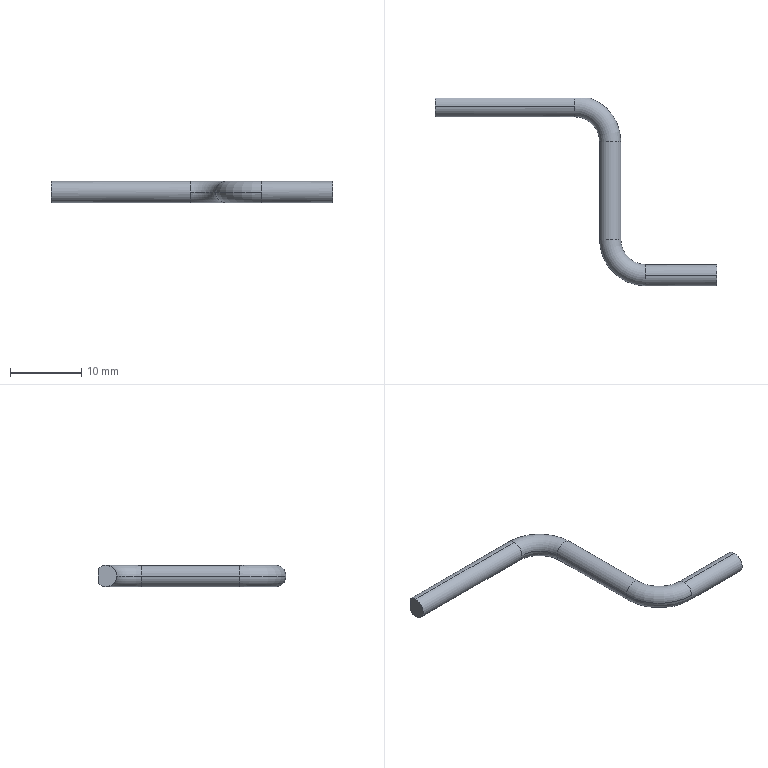Part | SolidWorks | features BaseBody 1 | 1 solid | 14 faces | box 39.607 x 26.395 x 3 mm | volume 406.832 mm3 | cylinder 7 | torus 4 | plane 3 | commonest cylinder face diameters 3 x7
STEP:
#1=CARTESIAN_POINT('',(-28.5,-35.,0.));
#2=VERTEX_POINT('',#1);
#3=CARTESIAN_POINT('',(-31.5,-35.,0.));
#4=VERTEX_POINT('',#3);
#5=CARTESIAN_POINT('',(-30.,-35.,0.));
#6=DIRECTION('',(0.,-1.,0.));
#7=DIRECTION('',(0.,0.,-1.));
#8=AXIS2_PLACEMENT_3D('',#5,#6,#7);
#9=CIRCLE('',#8,1.5);
#10=EDGE_CURVE('',#2,#4,#9,.T.);
#11=ORIENTED_EDGE('',*,*,#10,.T.);
#12=CARTESIAN_POINT('',(-25.,-41.5,0.));
#13=VERTEX_POINT('',#12);
#14=CARTESIAN_POINT('',(-25.,-35.,0.));
#15=DIRECTION('',(0.,0.,1.));
#16=DIRECTION('',(1.,0.,0.));
#17=AXIS2_PLACEMENT_3D('',#14,#15,#16);
#18=CIRCLE('',#17,6.5);
#19=EDGE_CURVE('',#4,#13,#18,.T.);
#20=ORIENTED_EDGE('',*,*,#19,.T.);
#21=CARTESIAN_POINT('',(-25.,-40.,1.5));
#22=VERTEX_POINT('',#21);
#23=CARTESIAN_POINT('',(-25.,-40.,0.));
#24=DIRECTION('',(1.,0.,0.));
#25=DIRECTION('',(0.,0.,-1.));
#26=AXIS2_PLACEMENT_3D('',#23,#24,#25);
#27=CIRCLE('',#26,1.5);
#28=EDGE_CURVE('',#22,#13,#27,.T.);
#29=ORIENTED_EDGE('',*,*,#28,.F.);
#30=CARTESIAN_POINT('',(-25.,-38.5,0.));
#31=VERTEX_POINT('',#30);
#32=CARTESIAN_POINT('',(-25.,-40.,0.));
#33=DIRECTION('',(1.,0.,0.));
#34=DIRECTION('',(0.,0.,-1.));
#35=AXIS2_PLACEMENT_3D('',#32,#33,#34);
#36=CIRCLE('',#35,1.5);
#37=EDGE_CURVE('',#31,#22,#36,.T.);
#38=ORIENTED_EDGE('',*,*,#37,.F.);
#39=CARTESIAN_POINT('',(-25.,-35.,0.));
#40=DIRECTION('',(0.,0.,1.));
#41=DIRECTION('',(1.,0.,0.));
#42=AXIS2_PLACEMENT_3D('',#39,#40,#41);
#43=CIRCLE('',#42,3.5);
#44=EDGE_CURVE('',#2,#31,#43,.T.);
#45=ORIENTED_EDGE('',*,*,#44,.F.);
#46=EDGE_LOOP('',(#11,#20,#29,#38,#45));
#47=FACE_OUTER_BOUND('',#46,.T.);
#48=CARTESIAN_POINT('',(-25.,-35.,0.));
#49=DIRECTION('',(0.,0.,1.));
#50=DIRECTION('',(1.,0.,0.));
#51=AXIS2_PLACEMENT_3D('',#48,#49,#50);
#52=TOROIDAL_SURFACE('',#51,5.,1.5);
#53=ADVANCED_FACE('',(#47),#52,.T.);
#54=CARTESIAN_POINT('',(-32.812,-15.105,0.));
#55=VERTEX_POINT('',#54);
#56=CARTESIAN_POINT('',(-35.,-15.105,-0.9972));
#57=VERTEX_POINT('',#56);
#58=CARTESIAN_POINT('',(-32.812,-15.105,0.));
#59=CARTESIAN_POINT('',(-32.812,-15.105,-0.1106));
#60=CARTESIAN_POINT('',(-32.849,-15.105,-0.2168));
#61=CARTESIAN_POINT('',(-32.968,-15.105,-0.4004));
#62=CARTESIAN_POINT('',(-33.048,-15.105,-0.4771));
#63=CARTESIAN_POINT('',(-33.31,-15.105,-0.6742));
#64=CARTESIAN_POINT('',(-33.512,-15.105,-0.76));
#65=CARTESIAN_POINT('',(-33.927,-15.105,-0.8892));
#66=CARTESIAN_POINT('',(-34.139,-15.105,-0.9304));
#67=CARTESIAN_POINT('',(-34.566,-15.105,-0.9846));
#68=CARTESIAN_POINT('',(-34.784,-15.105,-0.9972));
#69=CARTESIAN_POINT('',(-35.,-15.105,-0.9972));
#70=B_SPLINE_CURVE_WITH_KNOTS('',3,(#58,#59,#60,#61,#62,#63,#64,#65,#66,#67,#68,#69),.UNSPECIFIED.,.F.,.F.,(4,2,2,2,2,4),(0.,0.0003263,0.0006525,0.001305,0.001958,0.00261),.UNSPECIFIED.);
#71=EDGE_CURVE('',#55,#57,#70,.T.);
#72=ORIENTED_EDGE('',*,*,#71,.F.);
#73=CARTESIAN_POINT('',(-28.5,-21.225,0.));
#74=VERTEX_POINT('',#73);
#75=CARTESIAN_POINT('',(-35.,-21.225,0.));
#76=DIRECTION('',(0.,0.,-1.));
#77=DIRECTION('',(-1.,0.,0.));
#78=AXIS2_PLACEMENT_3D('',#75,#76,#77);
#79=CIRCLE('',#78,6.5);
#80=EDGE_CURVE('',#55,#74,#79,.T.);
#81=ORIENTED_EDGE('',*,*,#80,.T.);
#82=CARTESIAN_POINT('',(-31.5,-21.225,0.));
#83=VERTEX_POINT('',#82);
#84=CARTESIAN_POINT('',(-30.,-21.225,0.));
#85=DIRECTION('',(0.,-1.,0.));
#86=DIRECTION('',(0.,0.,-1.));
#87=AXIS2_PLACEMENT_3D('',#84,#85,#86);
#88=CIRCLE('',#87,1.5);
#89=EDGE_CURVE('',#83,#74,#88,.T.);
#90=ORIENTED_EDGE('',*,*,#89,.F.);
#91=CARTESIAN_POINT('',(-35.,-17.725,0.));
#92=VERTEX_POINT('',#91);
#93=CARTESIAN_POINT('',(-35.,-21.225,0.));
#94=DIRECTION('',(0.,0.,-1.));
#95=DIRECTION('',(-1.,0.,0.));
#96=AXIS2_PLACEMENT_3D('',#93,#94,#95);
#97=CIRCLE('',#96,3.5);
#98=EDGE_CURVE('',#92,#83,#97,.T.);
#99=ORIENTED_EDGE('',*,*,#98,.F.);
#100=CARTESIAN_POINT('',(-35.,-16.225,-1.5));
#101=VERTEX_POINT('',#100);
#102=CARTESIAN_POINT('',(-35.,-16.225,0.));
#103=DIRECTION('',(1.,0.,0.));
#104=DIRECTION('',(0.,0.,-1.));
#105=AXIS2_PLACEMENT_3D('',#102,#103,#104);
#106=CIRCLE('',#105,1.5);
#107=EDGE_CURVE('',#92,#101,#106,.T.);
#108=ORIENTED_EDGE('',*,*,#107,.T.);
#109=CARTESIAN_POINT('',(-35.,-16.225,0.));
#110=DIRECTION('',(1.,0.,0.));
#111=DIRECTION('',(0.,0.,-1.));
#112=AXIS2_PLACEMENT_3D('',#109,#110,#111);
#113=CIRCLE('',#112,1.5);
#114=EDGE_CURVE('',#101,#57,#113,.T.);
#115=ORIENTED_EDGE('',*,*,#114,.T.);
#116=EDGE_LOOP('',(#72,#81,#90,#99,#108,#115));
#117=FACE_OUTER_BOUND('',#116,.T.);
#118=CARTESIAN_POINT('',(-35.,-21.225,0.));
#119=DIRECTION('',(0.,0.,-1.));
#120=DIRECTION('',(-1.,0.,0.));
#121=AXIS2_PLACEMENT_3D('',#118,#119,#120);
#122=TOROIDAL_SURFACE('',#121,5.,1.5);
#123=ADVANCED_FACE('',(#117),#122,.T.);
#124=CARTESIAN_POINT('',(-25.,-40.,-1.5));
#125=VERTEX_POINT('',#124);
#126=CARTESIAN_POINT('',(-25.,-40.,0.));
#127=DIRECTION('',(1.,0.,0.));
#128=DIRECTION('',(0.,0.,-1.));
#129=AXIS2_PLACEMENT_3D('',#126,#127,#128);
#130=CIRCLE('',#129,1.5);
#131=EDGE_CURVE('',#125,#31,#130,.T.);
#132=ORIENTED_EDGE('',*,*,#131,.T.);
#133=ORIENTED_EDGE('',*,*,#37,.T.);
#134=CARTESIAN_POINT('',(-15.,-40.,1.5));
#135=VERTEX_POINT('',#134);
#136=CARTESIAN_POINT('',(-25.,-40.,1.5));
#137=DIRECTION('',(1.,0.,0.));
#138=VECTOR('',#137,1000.);
#139=LINE('',#136,#138);
#140=EDGE_CURVE('',#22,#135,#139,.T.);
#141=ORIENTED_EDGE('',*,*,#140,.T.);
#142=CARTESIAN_POINT('',(-15.,-40.,-1.5));
#143=VERTEX_POINT('',#142);
#144=CARTESIAN_POINT('',(-15.,-40.,0.));
#145=DIRECTION('',(1.,0.,0.));
#146=DIRECTION('',(0.,0.,-1.));
#147=AXIS2_PLACEMENT_3D('',#144,#145,#146);
#148=CIRCLE('',#147,1.5);
#149=EDGE_CURVE('',#143,#135,#148,.T.);
#150=ORIENTED_EDGE('',*,*,#149,.F.);
#151=CARTESIAN_POINT('',(-25.,-40.,-1.5));
#152=DIRECTION('',(1.,0.,0.));
#153=VECTOR('',#152,1000.);
#154=LINE('',#151,#153);
#155=EDGE_CURVE('',#125,#143,#154,.T.);
#156=ORIENTED_EDGE('',*,*,#155,.F.);
#157=EDGE_LOOP('',(#132,#133,#141,#150,#156));
#158=FACE_OUTER_BOUND('',#157,.T.);
#159=CARTESIAN_POINT('',(-25.,-40.,0.));
#160=DIRECTION('',(1.,0.,0.));
#161=DIRECTION('',(0.,0.,-1.));
#162=AXIS2_PLACEMENT_3D('',#159,#160,#161);
#163=CYLINDRICAL_SURFACE('',#162,1.5);
#164=ADVANCED_FACE('',(#158),#163,.T.);
#165=CARTESIAN_POINT('',(-30.,-21.225,0.));
#166=DIRECTION('',(0.,-1.,0.));
#167=DIRECTION('',(0.,0.,-1.));
#168=AXIS2_PLACEMENT_3D('',#165,#166,#167);
#169=CIRCLE('',#168,1.5);
#170=EDGE_CURVE('',#74,#83,#169,.T.);
#171=ORIENTED_EDGE('',*,*,#170,.T.);
#172=CARTESIAN_POINT('',(-31.5,-21.225,0.));
#173=DIRECTION('',(0.,-1.,0.));
#174=VECTOR('',#173,1000.);
#175=LINE('',#172,#174);
#176=EDGE_CURVE('',#83,#4,#175,.T.);
#177=ORIENTED_EDGE('',*,*,#176,.T.);
#178=ORIENTED_EDGE('',*,*,#10,.F.);
#179=CARTESIAN_POINT('',(-28.5,-21.225,0.));
#180=DIRECTION('',(0.,-1.,0.));
#181=VECTOR('',#180,1000.);
#182=LINE('',#179,#181);
#183=EDGE_CURVE('',#74,#2,#182,.T.);
#184=ORIENTED_EDGE('',*,*,#183,.F.);
#185=EDGE_LOOP('',(#171,#177,#178,#184));
#186=FACE_OUTER_BOUND('',#185,.T.);
#187=CARTESIAN_POINT('',(-30.,-21.225,0.));
#188=DIRECTION('',(0.,-1.,0.));
#189=DIRECTION('',(1.,0.,0.));
#190=AXIS2_PLACEMENT_3D('',#187,#188,#189);
#191=CYLINDRICAL_SURFACE('',#190,1.5);
#192=ADVANCED_FACE('',(#186),#191,.T.);
#193=CARTESIAN_POINT('',(-54.607,-15.105,0.9972));
#194=VERTEX_POINT('',#193);
#195=CARTESIAN_POINT('',(-54.607,-16.225,1.5));
#196=VERTEX_POINT('',#195);
#197=CARTESIAN_POINT('',(-54.607,-16.225,0.));
#198=DIRECTION('',(1.,0.,0.));
#199=DIRECTION('',(0.,0.,-1.));
#200=AXIS2_PLACEMENT_3D('',#197,#198,#199);
#201=CIRCLE('',#200,1.5);
#202=EDGE_CURVE('',#194,#196,#201,.T.);
#203=ORIENTED_EDGE('',*,*,#202,.T.);
#204=CARTESIAN_POINT('',(-35.,-16.225,1.5));
#205=VERTEX_POINT('',#204);
#206=CARTESIAN_POINT('',(-54.607,-16.225,1.5));
#207=DIRECTION('',(1.,0.,0.));
#208=VECTOR('',#207,1000.);
#209=LINE('',#206,#208);
#210=EDGE_CURVE('',#196,#205,#209,.T.);
#211=ORIENTED_EDGE('',*,*,#210,.T.);
#212=CARTESIAN_POINT('',(-35.,-15.105,0.9972));
#213=VERTEX_POINT('',#212);
#214=CARTESIAN_POINT('',(-35.,-16.225,0.));
#215=DIRECTION('',(1.,0.,0.));
#216=DIRECTION('',(0.,0.,-1.));
#217=AXIS2_PLACEMENT_3D('',#214,#215,#216);
#218=CIRCLE('',#217,1.5);
#219=EDGE_CURVE('',#213,#205,#218,.T.);
#220=ORIENTED_EDGE('',*,*,#219,.F.);
#221=CARTESIAN_POINT('',(-54.607,-15.105,0.9972));
#222=DIRECTION('',(1.,0.,0.));
#223=VECTOR('',#222,1000.);
#224=LINE('',#221,#223);
#225=EDGE_CURVE('',#194,#213,#224,.T.);
#226=ORIENTED_EDGE('',*,*,#225,.F.);
#227=EDGE_LOOP('',(#203,#211,#220,#226));
#228=FACE_OUTER_BOUND('',#227,.T.);
#229=CARTESIAN_POINT('',(-54.607,-16.225,0.));
#230=DIRECTION('',(1.,0.,0.));
#231=DIRECTION('',(0.,0.,-1.));
#232=AXIS2_PLACEMENT_3D('',#229,#230,#231);
#233=CYLINDRICAL_SURFACE('',#232,1.5);
#234=ADVANCED_FACE('',(#228),#233,.T.);
#235=ORIENTED_EDGE('',*,*,#210,.F.);
#236=CARTESIAN_POINT('',(-54.607,-16.225,-1.5));
#237=VERTEX_POINT('',#236);
#238=CARTESIAN_POINT('',(-54.607,-16.225,0.));
#239=DIRECTION('',(1.,0.,0.));
#240=DIRECTION('',(0.,0.,-1.));
#241=AXIS2_PLACEMENT_3D('',#238,#239,#240);
#242=CIRCLE('',#241,1.5);
#243=EDGE_CURVE('',#196,#237,#242,.T.);
#244=ORIENTED_EDGE('',*,*,#243,.T.);
#245=CARTESIAN_POINT('',(-54.607,-16.225,-1.5));
#246=DIRECTION('',(1.,0.,0.));
#247=VECTOR('',#246,1000.);
#248=LINE('',#245,#247);
#249=EDGE_CURVE('',#237,#101,#248,.T.);
#250=ORIENTED_EDGE('',*,*,#249,.T.);
#251=ORIENTED_EDGE('',*,*,#107,.F.);
#252=CARTESIAN_POINT('',(-35.,-16.225,0.));
#253=DIRECTION('',(1.,0.,0.));
#254=DIRECTION('',(0.,0.,-1.));
#255=AXIS2_PLACEMENT_3D('',#252,#253,#254);
#256=CIRCLE('',#255,1.5);
#257=EDGE_CURVE('',#205,#92,#256,.T.);
#258=ORIENTED_EDGE('',*,*,#257,.F.);
#259=EDGE_LOOP('',(#235,#244,#250,#251,#258));
#260=FACE_OUTER_BOUND('',#259,.T.);
#261=CARTESIAN_POINT('',(-54.607,-16.225,0.));
#262=DIRECTION('',(1.,0.,0.));
#263=DIRECTION('',(0.,0.,-1.));
#264=AXIS2_PLACEMENT_3D('',#261,#262,#263);
#265=CYLINDRICAL_SURFACE('',#264,1.5);
#266=ADVANCED_FACE('',(#260),#265,.T.);
#267=ORIENTED_EDGE('',*,*,#202,.F.);
#268=CARTESIAN_POINT('',(-54.607,-15.105,-0.9972));
#269=VERTEX_POINT('',#268);
#270=CARTESIAN_POINT('',(-54.607,-15.105,0.));
#271=DIRECTION('',(0.,0.,-1.));
#272=VECTOR('',#271,1000.);
#273=LINE('',#270,#272);
#274=EDGE_CURVE('',#194,#269,#273,.T.);
#275=ORIENTED_EDGE('',*,*,#274,.T.);
#276=CARTESIAN_POINT('',(-54.607,-16.225,0.));
#277=DIRECTION('',(1.,0.,0.));
#278=DIRECTION('',(0.,0.,-1.));
#279=AXIS2_PLACEMENT_3D('',#276,#277,#278);
#280=CIRCLE('',#279,1.5);
#281=EDGE_CURVE('',#237,#269,#280,.T.);
#282=ORIENTED_EDGE('',*,*,#281,.F.);
#283=ORIENTED_EDGE('',*,*,#243,.F.);
#284=EDGE_LOOP('',(#267,#275,#282,#283));
#285=FACE_OUTER_BOUND('',#284,.T.);
#286=CARTESIAN_POINT('',(-54.607,-16.225,0.));
#287=DIRECTION('',(1.,0.,0.));
#288=DIRECTION('',(0.,0.,-1.));
#289=AXIS2_PLACEMENT_3D('',#286,#287,#288);
#290=PLANE('',#289);
#291=ADVANCED_FACE('',(#285),#290,.F.);
#292=ORIENTED_EDGE('',*,*,#149,.T.);
#293=CARTESIAN_POINT('',(-15.,-40.,0.));
#294=DIRECTION('',(1.,0.,0.));
#295=DIRECTION('',(0.,0.,-1.));
#296=AXIS2_PLACEMENT_3D('',#293,#294,#295);
#297=CIRCLE('',#296,1.5);
#298=EDGE_CURVE('',#135,#143,#297,.T.);
#299=ORIENTED_EDGE('',*,*,#298,.T.);
#300=EDGE_LOOP('',(#292,#299));
#301=FACE_OUTER_BOUND('',#300,.T.);
#302=CARTESIAN_POINT('',(-15.,-40.,0.));
#303=DIRECTION('',(1.,0.,0.));
#304=DIRECTION('',(0.,0.,-1.));
#305=AXIS2_PLACEMENT_3D('',#302,#303,#304);
#306=PLANE('',#305);
#307=ADVANCED_FACE('',(#301),#306,.T.);
#308=ORIENTED_EDGE('',*,*,#249,.F.);
#309=ORIENTED_EDGE('',*,*,#281,.T.);
#310=CARTESIAN_POINT('',(-54.607,-15.105,-0.9972));
#311=DIRECTION('',(-1.,0.,0.));
#312=VECTOR('',#311,1000.);
#313=LINE('',#310,#312);
#314=EDGE_CURVE('',#57,#269,#313,.T.);
#315=ORIENTED_EDGE('',*,*,#314,.F.);
#316=ORIENTED_EDGE('',*,*,#114,.F.);
#317=EDGE_LOOP('',(#308,#309,#315,#316));
#318=FACE_OUTER_BOUND('',#317,.T.);
#319=CARTESIAN_POINT('',(-54.607,-16.225,0.));
#320=DIRECTION('',(1.,0.,0.));
#321=DIRECTION('',(0.,0.,-1.));
#322=AXIS2_PLACEMENT_3D('',#319,#320,#321);
#323=CYLINDRICAL_SURFACE('',#322,1.5);
#324=ADVANCED_FACE('',(#318),#323,.T.);
#325=ORIENTED_EDGE('',*,*,#80,.F.);
#326=CARTESIAN_POINT('',(-35.,-15.105,0.9972));
#327=CARTESIAN_POINT('',(-34.784,-15.105,0.9972));
#328=CARTESIAN_POINT('',(-34.567,-15.105,0.9846));
#329=CARTESIAN_POINT('',(-34.138,-15.105,0.9302));
#330=CARTESIAN_POINT('',(-33.925,-15.105,0.8888));
#331=CARTESIAN_POINT('',(-33.614,-15.105,0.7915));
#332=CARTESIAN_POINT('',(-33.512,-15.105,0.7535));
#333=CARTESIAN_POINT('',(-33.316,-15.105,0.6614));
#334=CARTESIAN_POINT('',(-33.22,-15.105,0.607));
#335=CARTESIAN_POINT('',(-33.047,-15.105,0.4769));
#336=CARTESIAN_POINT('',(-32.968,-15.105,0.3994));
#337=CARTESIAN_POINT('',(-32.849,-15.105,0.2172));
#338=CARTESIAN_POINT('',(-32.812,-15.105,0.1101));
#339=CARTESIAN_POINT('',(-32.812,-15.105,0.));
#340=B_SPLINE_CURVE_WITH_KNOTS('',3,(#326,#327,#328,#329,#330,#331,#332,#333,#334,#335,#336,#337,#338,#339),.UNSPECIFIED.,.F.,.F.,(4,2,2,2,2,2,4),(0.007822,0.008472,0.009122,0.009446,0.009771,0.0101,0.01042),.UNSPECIFIED.);
#341=EDGE_CURVE('',#213,#55,#340,.T.);
#342=ORIENTED_EDGE('',*,*,#341,.F.);
#343=ORIENTED_EDGE('',*,*,#219,.T.);
#344=ORIENTED_EDGE('',*,*,#257,.T.);
#345=ORIENTED_EDGE('',*,*,#98,.T.);
#346=ORIENTED_EDGE('',*,*,#170,.F.);
#347=EDGE_LOOP('',(#325,#342,#343,#344,#345,#346));
#348=FACE_OUTER_BOUND('',#347,.T.);
#349=CARTESIAN_POINT('',(-35.,-21.225,0.));
#350=DIRECTION('',(0.,0.,-1.));
#351=DIRECTION('',(-1.,0.,0.));
#352=AXIS2_PLACEMENT_3D('',#349,#350,#351);
#353=TOROIDAL_SURFACE('',#352,5.,1.5);
#354=ADVANCED_FACE('',(#348),#353,.T.);
#355=ORIENTED_EDGE('',*,*,#176,.F.);
#356=ORIENTED_EDGE('',*,*,#89,.T.);
#357=ORIENTED_EDGE('',*,*,#183,.T.);
#358=CARTESIAN_POINT('',(-30.,-35.,0.));
#359=DIRECTION('',(0.,-1.,0.));
#360=DIRECTION('',(0.,0.,-1.));
#361=AXIS2_PLACEMENT_3D('',#358,#359,#360);
#362=CIRCLE('',#361,1.5);
#363=EDGE_CURVE('',#4,#2,#362,.T.);
#364=ORIENTED_EDGE('',*,*,#363,.F.);
#365=EDGE_LOOP('',(#355,#356,#357,#364));
#366=FACE_OUTER_BOUND('',#365,.T.);
#367=CARTESIAN_POINT('',(-30.,-21.225,0.));
#368=DIRECTION('',(0.,-1.,0.));
#369=DIRECTION('',(1.,0.,0.));
#370=AXIS2_PLACEMENT_3D('',#367,#368,#369);
#371=CYLINDRICAL_SURFACE('',#370,1.5);
#372=ADVANCED_FACE('',(#366),#371,.T.);
#373=ORIENTED_EDGE('',*,*,#19,.F.);
#374=ORIENTED_EDGE('',*,*,#363,.T.);
#375=ORIENTED_EDGE('',*,*,#44,.T.);
#376=ORIENTED_EDGE('',*,*,#131,.F.);
#377=CARTESIAN_POINT('',(-25.,-40.,0.));
#378=DIRECTION('',(1.,0.,0.));
#379=DIRECTION('',(0.,0.,-1.));
#380=AXIS2_PLACEMENT_3D('',#377,#378,#379);
#381=CIRCLE('',#380,1.5);
#382=EDGE_CURVE('',#13,#125,#381,.T.);
#383=ORIENTED_EDGE('',*,*,#382,.F.);
#384=EDGE_LOOP('',(#373,#374,#375,#376,#383));
#385=FACE_OUTER_BOUND('',#384,.T.);
#386=CARTESIAN_POINT('',(-25.,-35.,0.));
#387=DIRECTION('',(0.,0.,1.));
#388=DIRECTION('',(1.,0.,0.));
#389=AXIS2_PLACEMENT_3D('',#386,#387,#388);
#390=TOROIDAL_SURFACE('',#389,5.,1.5);
#391=ADVANCED_FACE('',(#385),#390,.T.);
#392=ORIENTED_EDGE('',*,*,#140,.F.);
#393=ORIENTED_EDGE('',*,*,#28,.T.);
#394=ORIENTED_EDGE('',*,*,#382,.T.);
#395=ORIENTED_EDGE('',*,*,#155,.T.);
#396=ORIENTED_EDGE('',*,*,#298,.F.);
#397=EDGE_LOOP('',(#392,#393,#394,#395,#396));
#398=FACE_OUTER_BOUND('',#397,.T.);
#399=CARTESIAN_POINT('',(-25.,-40.,0.));
#400=DIRECTION('',(1.,0.,0.));
#401=DIRECTION('',(0.,0.,-1.));
#402=AXIS2_PLACEMENT_3D('',#399,#400,#401);
#403=CYLINDRICAL_SURFACE('',#402,1.5);
#404=ADVANCED_FACE('',(#398),#403,.T.);
#405=ORIENTED_EDGE('',*,*,#225,.T.);
#406=ORIENTED_EDGE('',*,*,#341,.T.);
#407=ORIENTED_EDGE('',*,*,#71,.T.);
#408=ORIENTED_EDGE('',*,*,#314,.T.);
#409=ORIENTED_EDGE('',*,*,#274,.F.);
#410=EDGE_LOOP('',(#405,#406,#407,#408,#409));
#411=FACE_OUTER_BOUND('',#410,.T.);
#412=CARTESIAN_POINT('',(-166.282,-15.105,-5.));
#413=DIRECTION('',(0.,-1.,0.));
#414=DIRECTION('',(0.,0.,-1.));
#415=AXIS2_PLACEMENT_3D('',#412,#413,#414);
#416=PLANE('',#415);
#417=ADVANCED_FACE('',(#411),#416,.F.);
#418=CLOSED_SHELL('',(#53,#123,#164,#192,#234,#266,#291,#307,#324,#354,#372,#391,#404,#417));
#419=MANIFOLD_SOLID_BREP('',#418);
#420=CARTESIAN_POINT('',(0.,0.,0.));
#421=DIRECTION('',(0.,0.,1.));
#422=DIRECTION('',(1.,0.,0.));
#423=AXIS2_PLACEMENT_3D('',#420,#421,#422);
#424=(LENGTH_UNIT()NAMED_UNIT(*)SI_UNIT(.MILLI.,.METRE.));
#425=UNCERTAINTY_MEASURE_WITH_UNIT(LENGTH_MEASURE(0.00001),#424,'','');
#426=(NAMED_UNIT(*)PLANE_ANGLE_UNIT()SI_UNIT($,.RADIAN.));
#427=(NAMED_UNIT(*)SI_UNIT($,.STERADIAN.)SOLID_ANGLE_UNIT());
#428=(GEOMETRIC_REPRESENTATION_CONTEXT(3)GLOBAL_UNCERTAINTY_ASSIGNED_CONTEXT((#425))GLOBAL_UNIT_ASSIGNED_CONTEXT((#424,#426,#427))REPRESENTATION_CONTEXT('',''));
#429=ADVANCED_BREP_SHAPE_REPRESENTATION('',(#419,#423),#428);